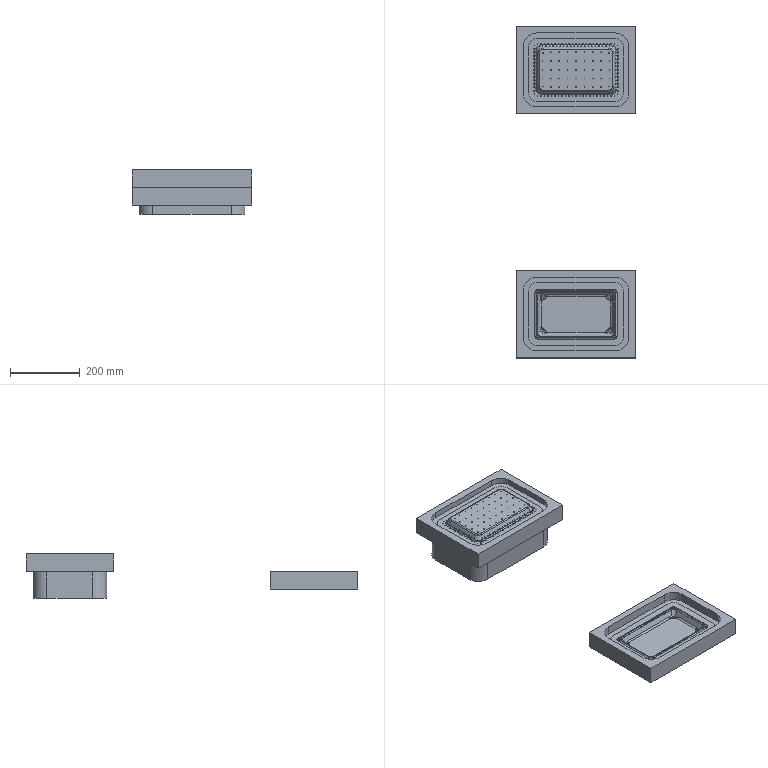Part | 7 solids | 1009 faces | box 343.99 x 952.259 x 127.368 mm | volume 5364463 mm3 | cylinder 495 | spline 252 | plane 238 | torus 24 | commonest cylinder face diameters 2 x191 1 x160 8 x24 8.588 x24 49.166 x20 79.166 x16